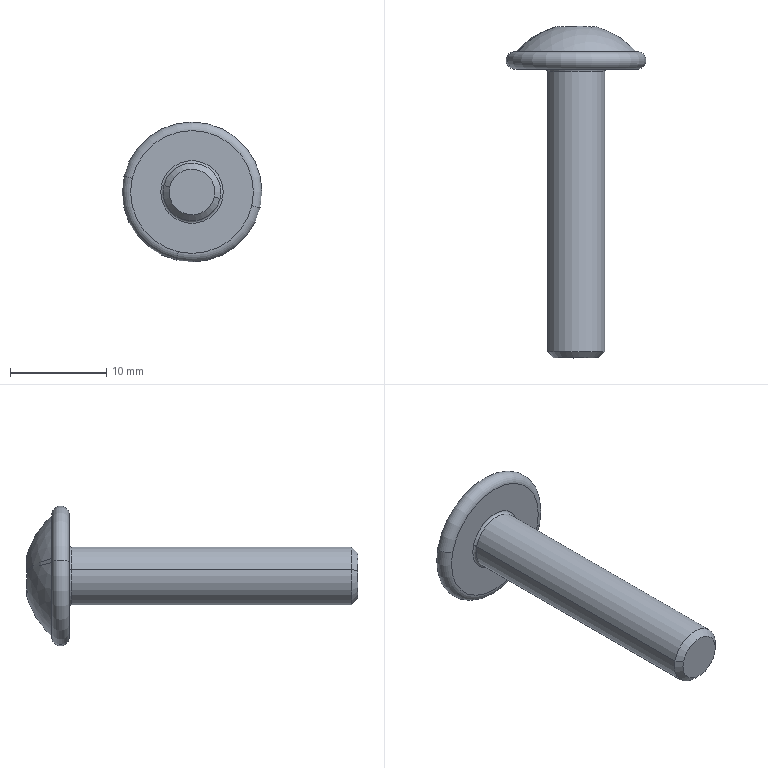Part | SolidWorks | features BaseBody 1 | 1 solid | 32 faces | box 14.55 x 34.479 x 14.55 mm | volume 1284 mm3 | cylinder 17 | torus 5 | sphere 4 | plane 4 | cone 2 | commonest cylinder face diameters 1.32 x6 3.14 x4 1 x3 1.26 x2 6 x2
STEP:
#1=CARTESIAN_POINT('',(1914.278,173.093,821.946));
#2=VERTEX_POINT('',#1);
#3=CARTESIAN_POINT('',(1913.973,173.055,822.157));
#4=VERTEX_POINT('',#3);
#5=CARTESIAN_POINT('',(1914.278,173.093,821.946));
#6=CARTESIAN_POINT('',(1914.154,173.093,821.975));
#7=CARTESIAN_POINT('',(1914.043,173.079,822.052));
#8=CARTESIAN_POINT('',(1913.973,173.055,822.157));
#9=B_SPLINE_CURVE_WITH_KNOTS('',3,(#5,#6,#7,#8),.UNSPECIFIED.,.F.,.F.,(4,4),(0.0003802,0.00076),.UNSPECIFIED.);
#10=EDGE_CURVE('',#2,#4,#9,.T.);
#11=ORIENTED_EDGE('',*,*,#10,.F.);
#12=CARTESIAN_POINT('',(1914.278,170.764,821.946));
#13=VERTEX_POINT('',#12);
#14=CARTESIAN_POINT('',(1914.278,173.214,821.946));
#15=DIRECTION('',(0.,-1.,0.));
#16=VECTOR('',#15,1000.);
#17=LINE('',#14,#16);
#18=EDGE_CURVE('',#2,#13,#17,.T.);
#19=ORIENTED_EDGE('',*,*,#18,.T.);
#20=CARTESIAN_POINT('',(1913.973,170.764,822.157));
#21=VERTEX_POINT('',#20);
#22=CARTESIAN_POINT('',(1914.39,170.764,822.434));
#23=DIRECTION('',(0.,-1.,0.));
#24=DIRECTION('',(-0.8332,0.,-0.5529));
#25=AXIS2_PLACEMENT_3D('',#22,#23,#24);
#26=CIRCLE('',#25,0.5);
#27=EDGE_CURVE('',#21,#13,#26,.T.);
#28=ORIENTED_EDGE('',*,*,#27,.F.);
#29=CARTESIAN_POINT('',(1913.973,170.764,822.157));
#30=DIRECTION('',(0.,1.,0.));
#31=VECTOR('',#30,1000.);
#32=LINE('',#29,#31);
#33=EDGE_CURVE('',#21,#4,#32,.T.);
#34=ORIENTED_EDGE('',*,*,#33,.T.);
#35=EDGE_LOOP('',(#11,#19,#28,#34));
#36=FACE_OUTER_BOUND('',#35,.T.);
#37=CARTESIAN_POINT('',(1914.39,173.214,822.434));
#38=DIRECTION('',(0.,-1.,0.));
#39=DIRECTION('',(-0.2239,0.,-0.9746));
#40=AXIS2_PLACEMENT_3D('',#37,#38,#39);
#41=CYLINDRICAL_SURFACE('',#40,0.5);
#42=ADVANCED_FACE('',(#36),#41,.T.);
#43=CARTESIAN_POINT('',(1912.656,172.978,818.453));
#44=VERTEX_POINT('',#43);
#45=CARTESIAN_POINT('',(1913.139,173.055,818.528));
#46=VERTEX_POINT('',#45);
#47=CARTESIAN_POINT('',(1912.656,172.978,818.453));
#48=CARTESIAN_POINT('',(1912.82,172.995,818.416));
#49=CARTESIAN_POINT('',(1912.995,173.023,818.443));
#50=CARTESIAN_POINT('',(1913.139,173.055,818.528));
#51=B_SPLINE_CURVE_WITH_KNOTS('',3,(#47,#48,#49,#50),.UNSPECIFIED.,.F.,.F.,(4,4),(0.0009315,0.001436),.UNSPECIFIED.);
#52=EDGE_CURVE('',#44,#46,#51,.T.);
#53=ORIENTED_EDGE('',*,*,#52,.F.);
#54=CARTESIAN_POINT('',(1912.656,170.764,818.453));
#55=VERTEX_POINT('',#54);
#56=CARTESIAN_POINT('',(1912.656,173.175,818.453));
#57=DIRECTION('',(0.,-1.,0.));
#58=VECTOR('',#57,1000.);
#59=LINE('',#56,#58);
#60=EDGE_CURVE('',#44,#55,#59,.T.);
#61=ORIENTED_EDGE('',*,*,#60,.T.);
#62=CARTESIAN_POINT('',(1913.139,170.764,818.528));
#63=VERTEX_POINT('',#62);
#64=CARTESIAN_POINT('',(1912.804,170.764,819.097));
#65=DIRECTION('',(0.,1.,0.));
#66=DIRECTION('',(0.5084,0.,-0.8611));
#67=AXIS2_PLACEMENT_3D('',#64,#65,#66);
#68=CIRCLE('',#67,0.66);
#69=EDGE_CURVE('',#63,#55,#68,.T.);
#70=ORIENTED_EDGE('',*,*,#69,.F.);
#71=CARTESIAN_POINT('',(1913.139,170.764,818.528));
#72=DIRECTION('',(0.,1.,0.));
#73=VECTOR('',#72,1000.);
#74=LINE('',#71,#73);
#75=EDGE_CURVE('',#63,#46,#74,.T.);
#76=ORIENTED_EDGE('',*,*,#75,.T.);
#77=EDGE_LOOP('',(#53,#61,#70,#76));
#78=FACE_OUTER_BOUND('',#77,.T.);
#79=CARTESIAN_POINT('',(1912.804,173.175,819.097));
#80=DIRECTION('',(0.,-1.,0.));
#81=DIRECTION('',(-0.2239,0.,-0.9746));
#82=AXIS2_PLACEMENT_3D('',#79,#80,#81);
#83=CYLINDRICAL_SURFACE('',#82,0.66);
#84=ADVANCED_FACE('',(#78),#83,.F.);
#85=CARTESIAN_POINT('',(1914.212,172.978,818.096));
#86=VERTEX_POINT('',#85);
#87=CARTESIAN_POINT('',(1914.972,173.009,818.492));
#88=VERTEX_POINT('',#87);
#89=CARTESIAN_POINT('',(1914.212,172.978,818.096));
#90=CARTESIAN_POINT('',(1914.363,172.962,818.061));
#91=CARTESIAN_POINT('',(1914.528,172.957,818.082));
#92=CARTESIAN_POINT('',(1914.804,172.968,818.226));
#93=CARTESIAN_POINT('',(1914.914,172.985,818.348));
#94=CARTESIAN_POINT('',(1914.972,173.009,818.492));
#95=B_SPLINE_CURVE_WITH_KNOTS('',3,(#89,#90,#91,#92,#93,#94),.UNSPECIFIED.,.F.,.F.,(4,2,4),(0.0005046,0.00097,0.001436),.UNSPECIFIED.);
#96=EDGE_CURVE('',#86,#88,#95,.T.);
#97=ORIENTED_EDGE('',*,*,#96,.F.);
#98=CARTESIAN_POINT('',(1914.212,170.764,818.096));
#99=VERTEX_POINT('',#98);
#100=CARTESIAN_POINT('',(1914.212,173.175,818.096));
#101=DIRECTION('',(0.,-1.,0.));
#102=VECTOR('',#101,1000.);
#103=LINE('',#100,#102);
#104=EDGE_CURVE('',#86,#99,#103,.T.);
#105=ORIENTED_EDGE('',*,*,#104,.T.);
#106=CARTESIAN_POINT('',(1914.972,170.764,818.492));
#107=VERTEX_POINT('',#106);
#108=CARTESIAN_POINT('',(1914.36,170.764,818.739));
#109=DIRECTION('',(0.,1.,0.));
#110=DIRECTION('',(0.9275,0.,-0.3739));
#111=AXIS2_PLACEMENT_3D('',#108,#109,#110);
#112=CIRCLE('',#111,0.66);
#113=EDGE_CURVE('',#107,#99,#112,.T.);
#114=ORIENTED_EDGE('',*,*,#113,.F.);
#115=CARTESIAN_POINT('',(1914.972,170.764,818.492));
#116=DIRECTION('',(0.,1.,0.));
#117=VECTOR('',#116,1000.);
#118=LINE('',#115,#117);
#119=EDGE_CURVE('',#107,#88,#118,.T.);
#120=ORIENTED_EDGE('',*,*,#119,.T.);
#121=EDGE_LOOP('',(#97,#105,#114,#120));
#122=FACE_OUTER_BOUND('',#121,.T.);
#123=CARTESIAN_POINT('',(1914.36,173.175,818.739));
#124=DIRECTION('',(0.,-1.,0.));
#125=DIRECTION('',(-0.2239,0.,-0.9746));
#126=AXIS2_PLACEMENT_3D('',#123,#124,#125);
#127=CYLINDRICAL_SURFACE('',#126,0.66);
#128=ADVANCED_FACE('',(#122),#127,.F.);
#129=CARTESIAN_POINT('',(1915.762,173.005,819.327));
#130=VERTEX_POINT('',#129);
#131=CARTESIAN_POINT('',(1916.054,172.959,819.608));
#132=VERTEX_POINT('',#131);
#133=CARTESIAN_POINT('',(1915.762,173.005,819.327));
#134=CARTESIAN_POINT('',(1915.887,172.983,819.386));
#135=CARTESIAN_POINT('',(1915.99,172.966,819.484));
#136=CARTESIAN_POINT('',(1916.054,172.959,819.608));
#137=B_SPLINE_CURVE_WITH_KNOTS('',3,(#133,#134,#135,#136),.UNSPECIFIED.,.F.,.F.,(4,4),(0.,0.0004132),.UNSPECIFIED.);
#138=EDGE_CURVE('',#130,#132,#137,.T.);
#139=ORIENTED_EDGE('',*,*,#138,.T.);
#140=CARTESIAN_POINT('',(1919.847,170.414,818.453));
#141=VERTEX_POINT('',#140);
#142=CARTESIAN_POINT('',(1913.892,165.077,820.266));
#143=DIRECTION('',(-0.2912,0.,-0.9567));
#144=DIRECTION('',(-0.9567,0.,0.2912));
#145=AXIS2_PLACEMENT_3D('',#142,#143,#144);
#146=CIRCLE('',#145,8.2);
#147=EDGE_CURVE('',#132,#141,#146,.T.);
#148=ORIENTED_EDGE('',*,*,#147,.T.);
#149=CARTESIAN_POINT('',(1907.825,170.414,821.659));
#150=VERTEX_POINT('',#149);
#151=CARTESIAN_POINT('',(1913.892,170.414,820.266));
#152=DIRECTION('',(0.,1.,0.));
#153=DIRECTION('',(0.9746,0.,-0.2239));
#154=AXIS2_PLACEMENT_3D('',#151,#152,#153);
#155=CIRCLE('',#154,6.225);
#156=EDGE_CURVE('',#141,#150,#155,.T.);
#157=ORIENTED_EDGE('',*,*,#156,.T.);
#158=CARTESIAN_POINT('',(1911.674,172.955,820.775));
#159=VERTEX_POINT('',#158);
#160=CARTESIAN_POINT('',(1913.892,165.077,820.266));
#161=DIRECTION('',(-0.2239,0.,-0.9746));
#162=DIRECTION('',(-0.7399,0.6509,0.1699));
#163=AXIS2_PLACEMENT_3D('',#160,#161,#162);
#164=CIRCLE('',#163,8.2);
#165=EDGE_CURVE('',#150,#159,#164,.T.);
#166=ORIENTED_EDGE('',*,*,#165,.T.);
#167=CARTESIAN_POINT('',(1911.799,173.005,820.237));
#168=VERTEX_POINT('',#167);
#169=CARTESIAN_POINT('',(1911.674,172.955,820.775));
#170=CARTESIAN_POINT('',(1911.631,172.955,820.587));
#171=CARTESIAN_POINT('',(1911.679,172.974,820.385));
#172=CARTESIAN_POINT('',(1911.799,173.005,820.237));
#173=B_SPLINE_CURVE_WITH_KNOTS('',3,(#169,#170,#171,#172),.UNSPECIFIED.,.F.,.F.,(4,4),(0.,0.0005707),.UNSPECIFIED.);
#174=EDGE_CURVE('',#159,#168,#173,.T.);
#175=ORIENTED_EDGE('',*,*,#174,.T.);
#176=CARTESIAN_POINT('',(1912.145,173.009,819.142));
#177=VERTEX_POINT('',#176);
#178=CARTESIAN_POINT('',(1911.799,173.005,820.237));
#179=CARTESIAN_POINT('',(1911.86,173.021,820.161));
#180=CARTESIAN_POINT('',(1911.914,173.033,820.08));
#181=CARTESIAN_POINT('',(1912.007,173.05,819.909));
#182=CARTESIAN_POINT('',(1912.046,173.054,819.817));
#183=CARTESIAN_POINT('',(1912.135,173.056,819.535));
#184=CARTESIAN_POINT('',(1912.159,173.04,819.338));
#185=CARTESIAN_POINT('',(1912.145,173.009,819.142));
#186=B_SPLINE_CURVE_WITH_KNOTS('',3,(#178,#179,#180,#181,#182,#183,#184,#185),.UNSPECIFIED.,.F.,.F.,(4,2,2,4),(0.,0.0002936,0.0005872,0.001174),.UNSPECIFIED.);
#187=EDGE_CURVE('',#168,#177,#186,.T.);
#188=ORIENTED_EDGE('',*,*,#187,.T.);
#189=CARTESIAN_POINT('',(1912.145,173.009,819.142));
#190=CARTESIAN_POINT('',(1912.135,172.985,818.987));
#191=CARTESIAN_POINT('',(1912.18,172.968,818.83));
#192=CARTESIAN_POINT('',(1912.366,172.957,818.578));
#193=CARTESIAN_POINT('',(1912.505,172.962,818.488));
#194=CARTESIAN_POINT('',(1912.656,172.978,818.453));
#195=B_SPLINE_CURVE_WITH_KNOTS('',3,(#189,#190,#191,#192,#193,#194),.UNSPECIFIED.,.F.,.F.,(4,2,4),(0.,0.0004658,0.0009315),.UNSPECIFIED.);
#196=EDGE_CURVE('',#177,#44,#195,.T.);
#197=ORIENTED_EDGE('',*,*,#196,.T.);
#198=ORIENTED_EDGE('',*,*,#52,.T.);
#199=CARTESIAN_POINT('',(1913.81,173.055,818.374));
#200=VERTEX_POINT('',#199);
#201=CARTESIAN_POINT('',(1913.139,173.055,818.528));
#202=CARTESIAN_POINT('',(1913.248,173.079,818.593));
#203=CARTESIAN_POINT('',(1913.382,173.093,818.614));
#204=CARTESIAN_POINT('',(1913.629,173.093,818.557));
#205=CARTESIAN_POINT('',(1913.74,173.079,818.479));
#206=CARTESIAN_POINT('',(1913.81,173.055,818.374));
#207=B_SPLINE_CURVE_WITH_KNOTS('',3,(#201,#202,#203,#204,#205,#206),.UNSPECIFIED.,.F.,.F.,(4,2,4),(0.,0.00038,0.00076),.UNSPECIFIED.);
#208=EDGE_CURVE('',#46,#200,#207,.T.);
#209=ORIENTED_EDGE('',*,*,#208,.T.);
#210=CARTESIAN_POINT('',(1913.81,173.055,818.374));
#211=CARTESIAN_POINT('',(1913.856,173.039,818.305));
#212=CARTESIAN_POINT('',(1913.915,173.024,818.245));
#213=CARTESIAN_POINT('',(1914.053,172.998,818.149));
#214=CARTESIAN_POINT('',(1914.13,172.986,818.115));
#215=CARTESIAN_POINT('',(1914.212,172.978,818.096));
#216=B_SPLINE_CURVE_WITH_KNOTS('',3,(#210,#211,#212,#213,#214,#215),.UNSPECIFIED.,.F.,.F.,(4,2,4),(0.,0.0002523,0.0005046),.UNSPECIFIED.);
#217=EDGE_CURVE('',#200,#86,#216,.T.);
#218=ORIENTED_EDGE('',*,*,#217,.T.);
#219=ORIENTED_EDGE('',*,*,#96,.T.);
#220=CARTESIAN_POINT('',(1914.972,173.009,818.492));
#221=CARTESIAN_POINT('',(1915.009,173.025,818.583));
#222=CARTESIAN_POINT('',(1915.054,173.036,818.67));
#223=CARTESIAN_POINT('',(1915.159,173.051,818.834));
#224=CARTESIAN_POINT('',(1915.22,173.055,818.913));
#225=CARTESIAN_POINT('',(1915.423,173.054,819.127));
#226=CARTESIAN_POINT('',(1915.585,173.037,819.244));
#227=CARTESIAN_POINT('',(1915.762,173.005,819.327));
#228=B_SPLINE_CURVE_WITH_KNOTS('',3,(#220,#221,#222,#223,#224,#225,#226,#227),.UNSPECIFIED.,.F.,.F.,(4,2,2,4),(0.,0.0002936,0.0005872,0.001174),.UNSPECIFIED.);
#229=EDGE_CURVE('',#88,#130,#228,.T.);
#230=ORIENTED_EDGE('',*,*,#229,.T.);
#231=EDGE_LOOP('',(#139,#148,#157,#166,#175,#188,#197,#198,#209,#218,#219,#230));
#232=FACE_OUTER_BOUND('',#231,.T.);
#233=CARTESIAN_POINT('',(1913.892,165.077,820.266));
#234=DIRECTION('',(-0.2912,0.,-0.9567));
#235=DIRECTION('',(-0.9567,0.,0.2912));
#236=AXIS2_PLACEMENT_3D('',#233,#234,#235);
#237=SPHERICAL_SURFACE('',#236,8.2);
#238=ADVANCED_FACE('',(#232),#237,.T.);
#239=CARTESIAN_POINT('',(1912.021,173.005,821.204));
#240=VERTEX_POINT('',#239);
#241=CARTESIAN_POINT('',(1911.729,172.959,820.924));
#242=VERTEX_POINT('',#241);
#243=CARTESIAN_POINT('',(1912.021,173.005,821.204));
#244=CARTESIAN_POINT('',(1911.896,172.983,821.146));
#245=CARTESIAN_POINT('',(1911.793,172.966,821.047));
#246=CARTESIAN_POINT('',(1911.729,172.959,820.924));
#247=B_SPLINE_CURVE_WITH_KNOTS('',3,(#243,#244,#245,#246),.UNSPECIFIED.,.F.,.F.,(4,4),(0.,0.0004132),.UNSPECIFIED.);
#248=EDGE_CURVE('',#240,#242,#247,.T.);
#249=ORIENTED_EDGE('',*,*,#248,.T.);
#250=CARTESIAN_POINT('',(1907.936,170.414,822.078));
#251=VERTEX_POINT('',#250);
#252=CARTESIAN_POINT('',(1913.892,165.077,820.266));
#253=DIRECTION('',(0.2912,0.,0.9567));
#254=DIRECTION('',(0.9567,0.,-0.2912));
#255=AXIS2_PLACEMENT_3D('',#252,#253,#254);
#256=CIRCLE('',#255,8.2);
#257=EDGE_CURVE('',#242,#251,#256,.T.);
#258=ORIENTED_EDGE('',*,*,#257,.T.);
#259=CARTESIAN_POINT('',(1919.959,170.414,818.872));
#260=VERTEX_POINT('',#259);
#261=CARTESIAN_POINT('',(1913.892,170.414,820.266));
#262=DIRECTION('',(0.,-1.,0.));
#263=DIRECTION('',(0.9746,0.,-0.2239));
#264=AXIS2_PLACEMENT_3D('',#261,#262,#263);
#265=CIRCLE('',#264,6.225);
#266=EDGE_CURVE('',#260,#251,#265,.T.);
#267=ORIENTED_EDGE('',*,*,#266,.F.);
#268=CARTESIAN_POINT('',(1916.109,172.955,819.756));
#269=VERTEX_POINT('',#268);
#270=CARTESIAN_POINT('',(1913.892,165.077,820.266));
#271=DIRECTION('',(-0.2239,0.,-0.9746));
#272=DIRECTION('',(0.7399,0.6509,-0.1699));
#273=AXIS2_PLACEMENT_3D('',#270,#271,#272);
#274=CIRCLE('',#273,8.2);
#275=EDGE_CURVE('',#269,#260,#274,.T.);
#276=ORIENTED_EDGE('',*,*,#275,.F.);
#277=CARTESIAN_POINT('',(1915.984,173.005,820.294));
#278=VERTEX_POINT('',#277);
#279=CARTESIAN_POINT('',(1916.109,172.955,819.756));
#280=CARTESIAN_POINT('',(1916.152,172.955,819.945));
#281=CARTESIAN_POINT('',(1916.104,172.974,820.146));
#282=CARTESIAN_POINT('',(1915.984,173.005,820.294));
#283=B_SPLINE_CURVE_WITH_KNOTS('',3,(#279,#280,#281,#282),.UNSPECIFIED.,.F.,.F.,(4,4),(0.,0.0005707),.UNSPECIFIED.);
#284=EDGE_CURVE('',#269,#278,#283,.T.);
#285=ORIENTED_EDGE('',*,*,#284,.T.);
#286=CARTESIAN_POINT('',(1915.638,173.009,821.39));
#287=VERTEX_POINT('',#286);
#288=CARTESIAN_POINT('',(1915.984,173.005,820.294));
#289=CARTESIAN_POINT('',(1915.923,173.021,820.37));
#290=CARTESIAN_POINT('',(1915.869,173.033,820.451));
#291=CARTESIAN_POINT('',(1915.776,173.05,820.623));
#292=CARTESIAN_POINT('',(1915.737,173.054,820.715));
#293=CARTESIAN_POINT('',(1915.648,173.056,820.996));
#294=CARTESIAN_POINT('',(1915.624,173.04,821.194));
#295=CARTESIAN_POINT('',(1915.638,173.009,821.39));
#296=B_SPLINE_CURVE_WITH_KNOTS('',3,(#288,#289,#290,#291,#292,#293,#294,#295),.UNSPECIFIED.,.F.,.F.,(4,2,2,4),(0.,0.0002936,0.0005872,0.001174),.UNSPECIFIED.);
#297=EDGE_CURVE('',#278,#287,#296,.T.);
#298=ORIENTED_EDGE('',*,*,#297,.T.);
#299=CARTESIAN_POINT('',(1914.644,173.055,822.003));
#300=VERTEX_POINT('',#299);
#301=CARTESIAN_POINT('',(1915.638,173.009,821.39));
#302=CARTESIAN_POINT('',(1915.646,172.991,821.509));
#303=CARTESIAN_POINT('',(1915.621,172.976,821.63));
#304=CARTESIAN_POINT('',(1915.512,172.96,821.842));
#305=CARTESIAN_POINT('',(1915.427,172.958,821.935));
#306=CARTESIAN_POINT('',(1915.222,172.968,822.06));
#307=CARTESIAN_POINT('',(1915.103,172.979,822.094));
#308=CARTESIAN_POINT('',(1914.864,173.012,822.096));
#309=CARTESIAN_POINT('',(1914.746,173.032,822.064));
#310=CARTESIAN_POINT('',(1914.644,173.055,822.003));
#311=B_SPLINE_CURVE_WITH_KNOTS('',3,(#301,#302,#303,#304,#305,#306,#307,#308,#309,#310),.UNSPECIFIED.,.F.,.F.,(4,2,2,2,4),(0.,0.0003589,0.0007178,0.001077,0.001436),.UNSPECIFIED.);
#312=EDGE_CURVE('',#287,#300,#311,.T.);
#313=ORIENTED_EDGE('',*,*,#312,.T.);
#314=CARTESIAN_POINT('',(1914.644,173.055,822.003));
#315=CARTESIAN_POINT('',(1914.535,173.079,821.939));
#316=CARTESIAN_POINT('',(1914.401,173.093,821.918));
#317=CARTESIAN_POINT('',(1914.278,173.093,821.946));
#318=B_SPLINE_CURVE_WITH_KNOTS('',3,(#314,#315,#316,#317),.UNSPECIFIED.,.F.,.F.,(4,4),(0.,0.0003802),.UNSPECIFIED.);
#319=EDGE_CURVE('',#300,#2,#318,.T.);
#320=ORIENTED_EDGE('',*,*,#319,.T.);
#321=ORIENTED_EDGE('',*,*,#10,.T.);
#322=CARTESIAN_POINT('',(1912.811,173.009,822.039));
#323=VERTEX_POINT('',#322);
#324=CARTESIAN_POINT('',(1913.973,173.055,822.157));
#325=CARTESIAN_POINT('',(1913.907,173.032,822.257));
#326=CARTESIAN_POINT('',(1913.815,173.012,822.336));
#327=CARTESIAN_POINT('',(1913.601,172.979,822.439));
#328=CARTESIAN_POINT('',(1913.478,172.968,822.461));
#329=CARTESIAN_POINT('',(1913.239,172.958,822.437));
#330=CARTESIAN_POINT('',(1913.123,172.96,822.392));
#331=CARTESIAN_POINT('',(1912.931,172.976,822.248));
#332=CARTESIAN_POINT('',(1912.856,172.991,822.15));
#333=CARTESIAN_POINT('',(1912.811,173.009,822.039));
#334=B_SPLINE_CURVE_WITH_KNOTS('',3,(#324,#325,#326,#327,#328,#329,#330,#331,#332,#333),.UNSPECIFIED.,.F.,.F.,(4,2,2,2,4),(0.,0.0003589,0.0007178,0.001077,0.001436),.UNSPECIFIED.);
#335=EDGE_CURVE('',#4,#323,#334,.T.);
#336=ORIENTED_EDGE('',*,*,#335,.T.);
#337=CARTESIAN_POINT('',(1912.811,173.009,822.039));
#338=CARTESIAN_POINT('',(1912.774,173.025,821.948));
#339=CARTESIAN_POINT('',(1912.729,173.036,821.862));
#340=CARTESIAN_POINT('',(1912.624,173.051,821.697));
#341=CARTESIAN_POINT('',(1912.563,173.055,821.618));
#342=CARTESIAN_POINT('',(1912.36,173.054,821.404));
#343=CARTESIAN_POINT('',(1912.198,173.037,821.288));
#344=CARTESIAN_POINT('',(1912.021,173.005,821.204));
#345=B_SPLINE_CURVE_WITH_KNOTS('',3,(#337,#338,#339,#340,#341,#342,#343,#344),.UNSPECIFIED.,.F.,.F.,(4,2,2,4),(0.,0.0002936,0.0005872,0.001174),.UNSPECIFIED.);
#346=EDGE_CURVE('',#323,#240,#345,.T.);
#347=ORIENTED_EDGE('',*,*,#346,.T.);
#348=EDGE_LOOP('',(#249,#258,#267,#276,#285,#298,#313,#320,#321,#336,#347));
#349=FACE_OUTER_BOUND('',#348,.T.);
#350=CARTESIAN_POINT('',(1913.892,165.077,820.266));
#351=DIRECTION('',(0.2912,0.,0.9567));
#352=DIRECTION('',(0.9567,0.,-0.2912));
#353=AXIS2_PLACEMENT_3D('',#350,#351,#352);
#354=SPHERICAL_SURFACE('',#353,8.2);
#355=ADVANCED_FACE('',(#349),#354,.T.);
#356=CARTESIAN_POINT('',(1912.464,170.414,814.053));
#357=VERTEX_POINT('',#356);
#358=CARTESIAN_POINT('',(1907.678,170.414,821.693));
#359=VERTEX_POINT('',#358);
#360=CARTESIAN_POINT('',(1913.892,170.414,820.266));
#361=DIRECTION('',(0.,1.,0.));
#362=DIRECTION('',(0.9746,0.,-0.2239));
#363=AXIS2_PLACEMENT_3D('',#360,#361,#362);
#364=CIRCLE('',#363,6.375);
#365=EDGE_CURVE('',#357,#359,#364,.T.);
#366=ORIENTED_EDGE('',*,*,#365,.F.);
#367=CARTESIAN_POINT('',(1912.464,168.614,814.053));
#368=VERTEX_POINT('',#367);
#369=CARTESIAN_POINT('',(1912.464,169.514,814.053));
#370=DIRECTION('',(-0.9746,0.,0.2239));
#371=DIRECTION('',(0.2239,0.,0.9746));
#372=AXIS2_PLACEMENT_3D('',#369,#370,#371);
#373=CIRCLE('',#372,0.9);
#374=EDGE_CURVE('',#357,#368,#373,.T.);
#375=ORIENTED_EDGE('',*,*,#374,.T.);
#376=CARTESIAN_POINT('',(1907.678,168.614,821.693));
#377=VERTEX_POINT('',#376);
#378=CARTESIAN_POINT('',(1913.892,168.614,820.266));
#379=DIRECTION('',(0.,1.,0.));
#380=DIRECTION('',(0.9746,0.,-0.2239));
#381=AXIS2_PLACEMENT_3D('',#378,#379,#380);
#382=CIRCLE('',#381,6.375);
#383=EDGE_CURVE('',#368,#377,#382,.T.);
#384=ORIENTED_EDGE('',*,*,#383,.T.);
#385=CARTESIAN_POINT('',(1907.678,169.514,821.693));
#386=DIRECTION('',(0.2239,0.,0.9746));
#387=DIRECTION('',(0.,-1.,0.));
#388=AXIS2_PLACEMENT_3D('',#385,#386,#387);
#389=CIRCLE('',#388,0.9);
#390=EDGE_CURVE('',#359,#377,#389,.T.);
#391=ORIENTED_EDGE('',*,*,#390,.F.);
#392=EDGE_LOOP('',(#366,#375,#384,#391));
#393=FACE_OUTER_BOUND('',#392,.T.);
#394=CARTESIAN_POINT('',(1913.892,169.514,820.266));
#395=DIRECTION('',(0.,-1.,0.));
#396=DIRECTION('',(-0.2239,0.,-0.9746));
#397=AXIS2_PLACEMENT_3D('',#394,#395,#396);
#398=TOROIDAL_SURFACE('',#397,6.375,0.9);
#399=ADVANCED_FACE('',(#393),#398,.T.);
#400=CARTESIAN_POINT('',(1916.206,138.614,819.734));
#401=VERTEX_POINT('',#400);
#402=CARTESIAN_POINT('',(1911.577,138.614,820.797));
#403=VERTEX_POINT('',#402);
#404=CARTESIAN_POINT('',(1913.892,138.614,820.266));
#405=DIRECTION('',(0.,-1.,0.));
#406=DIRECTION('',(0.9746,0.,-0.2239));
#407=AXIS2_PLACEMENT_3D('',#404,#405,#406);
#408=CIRCLE('',#407,2.375);
#409=EDGE_CURVE('',#401,#403,#408,.T.);
#410=ORIENTED_EDGE('',*,*,#409,.T.);
#411=CARTESIAN_POINT('',(1913.892,138.614,820.266));
#412=DIRECTION('',(0.,-1.,0.));
#413=DIRECTION('',(-0.9746,0.,0.2239));
#414=AXIS2_PLACEMENT_3D('',#411,#412,#413);
#415=CIRCLE('',#414,2.375);
#416=EDGE_CURVE('',#403,#401,#415,.T.);
#417=ORIENTED_EDGE('',*,*,#416,.T.);
#418=EDGE_LOOP('',(#410,#417));
#419=FACE_OUTER_BOUND('',#418,.T.);
#420=CARTESIAN_POINT('',(1916.882,138.614,822.139));
#421=DIRECTION('',(0.,-1.,0.));
#422=DIRECTION('',(-0.9746,0.,0.2239));
#423=AXIS2_PLACEMENT_3D('',#420,#421,#422);
#424=PLANE('',#423);
#425=ADVANCED_FACE('',(#419),#424,.T.);
#426=CARTESIAN_POINT('',(1910.968,139.239,820.937));
#427=VERTEX_POINT('',#426);
#428=CARTESIAN_POINT('',(1911.577,138.614,820.797));
#429=DIRECTION('',(-0.6892,0.7071,0.1583));
#430=VECTOR('',#429,1000.);
#431=LINE('',#428,#430);
#432=EDGE_CURVE('',#403,#427,#431,.T.);
#433=ORIENTED_EDGE('',*,*,#432,.T.);
#434=CARTESIAN_POINT('',(1916.815,139.239,819.594));
#435=VERTEX_POINT('',#434);
#436=CARTESIAN_POINT('',(1913.892,139.239,820.266));
#437=DIRECTION('',(0.,-1.,0.));
#438=DIRECTION('',(-0.9746,0.,0.2239));
#439=AXIS2_PLACEMENT_3D('',#436,#437,#438);
#440=CIRCLE('',#439,3.);
#441=EDGE_CURVE('',#427,#435,#440,.T.);
#442=ORIENTED_EDGE('',*,*,#441,.T.);
#443=CARTESIAN_POINT('',(1916.206,138.614,819.734));
#444=DIRECTION('',(-0.6892,-0.7071,0.1583));
#445=VECTOR('',#444,1000.);
#446=LINE('',#443,#445);
#447=EDGE_CURVE('',#435,#401,#446,.T.);
#448=ORIENTED_EDGE('',*,*,#447,.T.);
#449=ORIENTED_EDGE('',*,*,#416,.F.);
#450=EDGE_LOOP('',(#433,#442,#448,#449));
#451=FACE_OUTER_BOUND('',#450,.T.);
#452=CARTESIAN_POINT('',(1913.892,139.324,820.266));
#453=DIRECTION('',(0.,1.,0.));
#454=DIRECTION('',(-0.9746,0.,0.2239));
#455=AXIS2_PLACEMENT_3D('',#452,#453,#454);
#456=CONICAL_SURFACE('',#455,3.085,0.7854);
#457=ADVANCED_FACE('',(#451),#456,.T.);
#458=ORIENTED_EDGE('',*,*,#447,.F.);
#459=CARTESIAN_POINT('',(1913.892,139.239,820.266));
#460=DIRECTION('',(0.,-1.,0.));
#461=DIRECTION('',(0.9746,0.,-0.2239));
#462=AXIS2_PLACEMENT_3D('',#459,#460,#461);
#463=CIRCLE('',#462,3.);
#464=EDGE_CURVE('',#435,#427,#463,.T.);
#465=ORIENTED_EDGE('',*,*,#464,.T.);
#466=ORIENTED_EDGE('',*,*,#432,.F.);
#467=ORIENTED_EDGE('',*,*,#409,.F.);
#468=EDGE_LOOP('',(#458,#465,#466,#467));
#469=FACE_OUTER_BOUND('',#468,.T.);
#470=CARTESIAN_POINT('',(1913.892,139.324,820.266));
#471=DIRECTION('',(0.,1.,0.));
#472=DIRECTION('',(-0.9746,0.,0.2239));
#473=AXIS2_PLACEMENT_3D('',#470,#471,#472);
#474=CONICAL_SURFACE('',#473,3.085,0.7854);
#475=ADVANCED_FACE('',(#469),#474,.T.);
#476=CARTESIAN_POINT('',(1910.968,168.364,820.937));
#477=VERTEX_POINT('',#476);
#478=CARTESIAN_POINT('',(1910.968,168.364,820.937));
#479=DIRECTION('',(0.,1.,0.));
#480=VECTOR('',#479,1000.);
#481=LINE('',#478,#480);
#482=EDGE_CURVE('',#427,#477,#481,.T.);
#483=ORIENTED_EDGE('',*,*,#482,.F.);
#484=ORIENTED_EDGE('',*,*,#464,.F.);
#485=CARTESIAN_POINT('',(1916.815,168.364,819.594));
#486=VERTEX_POINT('',#485);
#487=CARTESIAN_POINT('',(1916.815,168.364,819.594));
#488=DIRECTION('',(0.,-1.,0.));
#489=VECTOR('',#488,1000.);
#490=LINE('',#487,#489);
#491=EDGE_CURVE('',#486,#435,#490,.T.);
#492=ORIENTED_EDGE('',*,*,#491,.F.);
#493=CARTESIAN_POINT('',(1913.892,168.364,820.266));
#494=DIRECTION('',(0.,-1.,0.));
#495=DIRECTION('',(0.9746,0.,-0.2239));
#496=AXIS2_PLACEMENT_3D('',#493,#494,#495);
#497=CIRCLE('',#496,3.);
#498=EDGE_CURVE('',#486,#477,#497,.T.);
#499=ORIENTED_EDGE('',*,*,#498,.T.);
#500=EDGE_LOOP('',(#483,#484,#492,#499));
#501=FACE_OUTER_BOUND('',#500,.T.);
#502=CARTESIAN_POINT('',(1913.892,168.947,820.266));
#503=DIRECTION('',(0.,-1.,0.));
#504=DIRECTION('',(0.9746,0.,-0.2239));
#505=AXIS2_PLACEMENT_3D('',#502,#503,#504);
#506=CYLINDRICAL_SURFACE('',#505,3.);
#507=ADVANCED_FACE('',(#501),#506,.T.);
#508=CARTESIAN_POINT('',(1910.724,168.614,820.993));
#509=VERTEX_POINT('',#508);
#510=CARTESIAN_POINT('',(1910.724,168.364,820.993));
#511=DIRECTION('',(0.2239,0.,0.9746));
#512=DIRECTION('',(0.000000004,1.,-0.000000001));
#513=AXIS2_PLACEMENT_3D('',#510,#511,#512);
#514=CIRCLE('',#513,0.25);
#515=EDGE_CURVE('',#477,#509,#514,.T.);
#516=ORIENTED_EDGE('',*,*,#515,.F.);
#517=ORIENTED_EDGE('',*,*,#498,.F.);
#518=CARTESIAN_POINT('',(1917.059,168.614,819.538));
#519=VERTEX_POINT('',#518);
#520=CARTESIAN_POINT('',(1917.059,168.364,819.538));
#521=DIRECTION('',(0.2239,0.,0.9746));
#522=DIRECTION('',(-0.000000004,1.,0.000000001));
#523=AXIS2_PLACEMENT_3D('',#520,#521,#522);
#524=CIRCLE('',#523,0.25);
#525=EDGE_CURVE('',#519,#486,#524,.T.);
#526=ORIENTED_EDGE('',*,*,#525,.F.);
#527=CARTESIAN_POINT('',(1913.892,168.614,820.266));
#528=DIRECTION('',(0.,-1.,0.));
#529=DIRECTION('',(0.9746,0.,-0.2239));
#530=AXIS2_PLACEMENT_3D('',#527,#528,#529);
#531=CIRCLE('',#530,3.25);
#532=EDGE_CURVE('',#519,#509,#531,.T.);
#533=ORIENTED_EDGE('',*,*,#532,.T.);
#534=EDGE_LOOP('',(#516,#517,#526,#533));
#535=FACE_OUTER_BOUND('',#534,.T.);
#536=CARTESIAN_POINT('',(1913.892,168.364,820.266));
#537=DIRECTION('',(0.,-1.,0.));
#538=DIRECTION('',(0.9746,0.,-0.2239));
#539=AXIS2_PLACEMENT_3D('',#536,#537,#538);
#540=TOROIDAL_SURFACE('',#539,3.25,0.25);
#541=ADVANCED_FACE('',(#535),#540,.F.);
#542=CARTESIAN_POINT('',(1920.105,168.614,818.839));
#543=VERTEX_POINT('',#542);
#544=CARTESIAN_POINT('',(1913.892,168.614,820.266));
#545=DIRECTION('',(0.,1.,0.));
#546=DIRECTION('',(0.9746,0.,-0.2239));
#547=AXIS2_PLACEMENT_3D('',#544,#545,#546);
#548=CIRCLE('',#547,6.375);
#549=EDGE_CURVE('',#543,#368,#548,.T.);
#550=ORIENTED_EDGE('',*,*,#549,.F.);
#551=CARTESIAN_POINT('',(1913.892,168.614,820.266));
#552=DIRECTION('',(0.,-1.,0.));
#553=DIRECTION('',(0.9746,0.,-0.2239));
#554=AXIS2_PLACEMENT_3D('',#551,#552,#553);
#555=CIRCLE('',#554,6.375);
#556=EDGE_CURVE('',#543,#377,#555,.T.);
#557=ORIENTED_EDGE('',*,*,#556,.T.);
#558=ORIENTED_EDGE('',*,*,#383,.F.);
#559=EDGE_LOOP('',(#550,#557,#558));
#560=FACE_OUTER_BOUND('',#559,.T.);
#561=CARTESIAN_POINT('',(1913.892,168.614,820.266));
#562=DIRECTION('',(0.,-1.,0.));
#563=DIRECTION('',(-0.9746,0.,0.2239));
#564=AXIS2_PLACEMENT_3D('',#561,#562,#563);
#565=CIRCLE('',#564,3.25);
#566=EDGE_CURVE('',#509,#519,#565,.T.);
#567=ORIENTED_EDGE('',*,*,#566,.F.);
#568=ORIENTED_EDGE('',*,*,#532,.F.);
#569=EDGE_LOOP('',(#567,#568));
#570=FACE_BOUND('',#569,.T.);
#571=CARTESIAN_POINT('',(1921.842,168.614,825.262));
#572=DIRECTION('',(0.,-1.,0.));
#573=DIRECTION('',(-0.9746,0.,0.2239));
#574=AXIS2_PLACEMENT_3D('',#571,#572,#573);
#575=PLANE('',#574);
#576=ADVANCED_FACE('',(#560,#570),#575,.T.);
#577=CARTESIAN_POINT('',(1920.105,170.414,818.839));
#578=VERTEX_POINT('',#577);
#579=CARTESIAN_POINT('',(1913.892,170.414,820.266));
#580=DIRECTION('',(0.,-1.,0.));
#581=DIRECTION('',(0.9746,0.,-0.2239));
#582=AXIS2_PLACEMENT_3D('',#579,#580,#581);
#583=CIRCLE('',#582,6.375);
#584=EDGE_CURVE('',#578,#359,#583,.T.);
#585=ORIENTED_EDGE('',*,*,#584,.T.);
#586=ORIENTED_EDGE('',*,*,#390,.T.);
#587=ORIENTED_EDGE('',*,*,#556,.F.);
#588=CARTESIAN_POINT('',(1920.105,169.514,818.839));
#589=DIRECTION('',(0.2239,0.,0.9746));
#590=DIRECTION('',(0.,-1.,0.));
#591=AXIS2_PLACEMENT_3D('',#588,#589,#590);
#592=CIRCLE('',#591,0.9);
#593=EDGE_CURVE('',#543,#578,#592,.T.);
#594=ORIENTED_EDGE('',*,*,#593,.T.);
#595=EDGE_LOOP('',(#585,#586,#587,#594));
#596=FACE_OUTER_BOUND('',#595,.T.);
#597=CARTESIAN_POINT('',(1913.892,169.514,820.266));
#598=DIRECTION('',(0.,-1.,0.));
#599=DIRECTION('',(-0.2239,0.,-0.9746));
#600=AXIS2_PLACEMENT_3D('',#597,#598,#599);
#601=TOROIDAL_SURFACE('',#600,6.375,0.9);
#602=ADVANCED_FACE('',(#596),#601,.T.);
#603=ORIENTED_EDGE('',*,*,#374,.F.);
#604=CARTESIAN_POINT('',(1913.892,170.414,820.266));
#605=DIRECTION('',(0.,1.,0.));
#606=DIRECTION('',(0.9746,0.,-0.2239));
#607=AXIS2_PLACEMENT_3D('',#604,#605,#606);
#608=CIRCLE('',#607,6.375);
#609=EDGE_CURVE('',#578,#357,#608,.T.);
#610=ORIENTED_EDGE('',*,*,#609,.F.);
#611=ORIENTED_EDGE('',*,*,#593,.F.);
#612=ORIENTED_EDGE('',*,*,#549,.T.);
#613=EDGE_LOOP('',(#603,#610,#611,#612));
#614=FACE_OUTER_BOUND('',#613,.T.);
#615=CARTESIAN_POINT('',(1913.892,169.514,820.266));
#616=DIRECTION('',(0.,-1.,0.));
#617=DIRECTION('',(-0.2239,0.,-0.9746));
#618=AXIS2_PLACEMENT_3D('',#615,#616,#617);
#619=TOROIDAL_SURFACE('',#618,6.375,0.9);
#620=ADVANCED_FACE('',(#614),#619,.T.);
#621=ORIENTED_EDGE('',*,*,#584,.F.);
#622=ORIENTED_EDGE('',*,*,#609,.T.);
#623=ORIENTED_EDGE('',*,*,#365,.T.);
#624=EDGE_LOOP('',(#621,#622,#623));
#625=FACE_OUTER_BOUND('',#624,.T.);
#626=CARTESIAN_POINT('',(1913.892,170.414,820.266));
#627=DIRECTION('',(0.,1.,0.));
#628=DIRECTION('',(0.9746,0.,-0.2239));
#629=AXIS2_PLACEMENT_3D('',#626,#627,#628);
#630=CIRCLE('',#629,6.225);
#631=EDGE_CURVE('',#260,#141,#630,.T.);
#632=ORIENTED_EDGE('',*,*,#631,.F.);
#633=ORIENTED_EDGE('',*,*,#266,.T.);
#634=CARTESIAN_POINT('',(1913.892,170.414,820.266));
#635=DIRECTION('',(0.,-1.,0.));
#636=DIRECTION('',(0.9746,0.,-0.2239));
#637=AXIS2_PLACEMENT_3D('',#634,#635,#636);
#638=CIRCLE('',#637,6.225);
#639=EDGE_CURVE('',#251,#150,#638,.T.);
#640=ORIENTED_EDGE('',*,*,#639,.T.);
#641=ORIENTED_EDGE('',*,*,#156,.F.);
#642=EDGE_LOOP('',(#632,#633,#640,#641));
#643=FACE_BOUND('',#642,.T.);
#644=CARTESIAN_POINT('',(1921.842,170.414,825.262));
#645=DIRECTION('',(0.,1.,0.));
#646=DIRECTION('',(-0.2239,0.,-0.9746));
#647=AXIS2_PLACEMENT_3D('',#644,#645,#646);
#648=PLANE('',#647);
#649=ADVANCED_FACE('',(#625,#643),#648,.T.);
#650=ORIENTED_EDGE('',*,*,#257,.F.);
#651=CARTESIAN_POINT('',(1911.729,172.959,820.924));
#652=CARTESIAN_POINT('',(1911.705,172.956,820.877));
#653=CARTESIAN_POINT('',(1911.686,172.955,820.827));
#654=CARTESIAN_POINT('',(1911.674,172.955,820.775));
#655=B_SPLINE_CURVE_WITH_KNOTS('',3,(#651,#652,#653,#654),.UNSPECIFIED.,.F.,.F.,(4,4),(0.0004132,0.0005707),.UNSPECIFIED.);
#656=EDGE_CURVE('',#242,#159,#655,.T.);
#657=ORIENTED_EDGE('',*,*,#656,.T.);
#658=ORIENTED_EDGE('',*,*,#165,.F.);
#659=ORIENTED_EDGE('',*,*,#639,.F.);
#660=EDGE_LOOP('',(#650,#657,#658,#659));
#661=FACE_OUTER_BOUND('',#660,.T.);
#662=CARTESIAN_POINT('',(1913.892,165.077,820.266));
#663=DIRECTION('',(0.2912,0.,0.9567));
#664=DIRECTION('',(0.9567,0.,-0.2912));
#665=AXIS2_PLACEMENT_3D('',#662,#663,#664);
#666=SPHERICAL_SURFACE('',#665,8.2);
#667=ADVANCED_FACE('',(#661),#666,.T.);
#668=CARTESIAN_POINT('',(1911.799,170.764,820.237));
#669=VERTEX_POINT('',#668);
#670=CARTESIAN_POINT('',(1912.021,170.764,821.204));
#671=VERTEX_POINT('',#670);
#672=CARTESIAN_POINT('',(1912.288,170.764,820.634));
#673=DIRECTION('',(0.,1.,0.));
#674=DIRECTION('',(-0.7769,0.,-0.6296));
#675=AXIS2_PLACEMENT_3D('',#672,#673,#674);
#676=CIRCLE('',#675,0.63);
#677=EDGE_CURVE('',#669,#671,#676,.T.);
#678=ORIENTED_EDGE('',*,*,#677,.F.);
#679=CARTESIAN_POINT('',(1911.799,170.764,820.237));
#680=DIRECTION('',(0.,1.,0.));
#681=VECTOR('',#680,1000.);
#682=LINE('',#679,#681);
#683=EDGE_CURVE('',#669,#168,#682,.T.);
#684=ORIENTED_EDGE('',*,*,#683,.T.);
#685=ORIENTED_EDGE('',*,*,#174,.F.);
#686=ORIENTED_EDGE('',*,*,#656,.F.);
#687=ORIENTED_EDGE('',*,*,#248,.F.);
#688=CARTESIAN_POINT('',(1912.021,170.764,821.204));
#689=DIRECTION('',(0.,1.,0.));
#690=VECTOR('',#689,1000.);
#691=LINE('',#688,#690);
#692=EDGE_CURVE('',#671,#240,#691,.T.);
#693=ORIENTED_EDGE('',*,*,#692,.F.);
#694=EDGE_LOOP('',(#678,#684,#685,#686,#687,#693));
#695=FACE_OUTER_BOUND('',#694,.T.);
#696=CARTESIAN_POINT('',(1912.288,173.125,820.634));
#697=DIRECTION('',(0.,-1.,0.));
#698=DIRECTION('',(-0.2239,0.,-0.9746));
#699=AXIS2_PLACEMENT_3D('',#696,#697,#698);
#700=CYLINDRICAL_SURFACE('',#699,0.63);
#701=ADVANCED_FACE('',(#695),#700,.F.);
#702=ORIENTED_EDGE('',*,*,#346,.F.);
#703=CARTESIAN_POINT('',(1912.811,170.764,822.039));
#704=VERTEX_POINT('',#703);
#705=CARTESIAN_POINT('',(1912.811,170.764,822.039));
#706=DIRECTION('',(0.,1.,0.));
#707=VECTOR('',#706,1000.);
#708=LINE('',#705,#707);
#709=EDGE_CURVE('',#704,#323,#708,.T.);
#710=ORIENTED_EDGE('',*,*,#709,.F.);
#711=CARTESIAN_POINT('',(1911.355,170.764,822.626));
#712=DIRECTION('',(0.,-1.,0.));
#713=DIRECTION('',(0.4243,0.,-0.9055));
#714=AXIS2_PLACEMENT_3D('',#711,#712,#713);
#715=CIRCLE('',#714,1.57);
#716=EDGE_CURVE('',#671,#704,#715,.T.);
#717=ORIENTED_EDGE('',*,*,#716,.F.);
#718=ORIENTED_EDGE('',*,*,#692,.T.);
#719=EDGE_LOOP('',(#702,#710,#717,#718));
#720=FACE_OUTER_BOUND('',#719,.T.);
#721=CARTESIAN_POINT('',(1911.355,173.175,822.626));
#722=DIRECTION('',(0.,-1.,0.));
#723=DIRECTION('',(-0.2239,0.,-0.9746));
#724=AXIS2_PLACEMENT_3D('',#721,#722,#723);
#725=CYLINDRICAL_SURFACE('',#724,1.57);
#726=ADVANCED_FACE('',(#720),#725,.T.);
#727=ORIENTED_EDGE('',*,*,#716,.T.);
#728=CARTESIAN_POINT('',(1913.423,170.764,821.792));
#729=DIRECTION('',(0.,1.,0.));
#730=DIRECTION('',(-0.9275,0.,0.3739));
#731=AXIS2_PLACEMENT_3D('',#728,#729,#730);
#732=CIRCLE('',#731,0.66);
#733=EDGE_CURVE('',#704,#21,#732,.T.);
#734=ORIENTED_EDGE('',*,*,#733,.T.);
#735=ORIENTED_EDGE('',*,*,#27,.T.);
#736=CARTESIAN_POINT('',(1914.644,170.764,822.003));
#737=VERTEX_POINT('',#736);
#738=CARTESIAN_POINT('',(1914.39,170.764,822.434));
#739=DIRECTION('',(0.,-1.,0.));
#740=DIRECTION('',(-0.8332,0.,-0.5529));
#741=AXIS2_PLACEMENT_3D('',#738,#739,#740);
#742=CIRCLE('',#741,0.5);
#743=EDGE_CURVE('',#13,#737,#742,.T.);
#744=ORIENTED_EDGE('',*,*,#743,.T.);
#745=CARTESIAN_POINT('',(1915.638,170.764,821.39));
#746=VERTEX_POINT('',#745);
#747=CARTESIAN_POINT('',(1914.979,170.764,821.435));
#748=DIRECTION('',(0.,1.,0.));
#749=DIRECTION('',(-0.5084,0.,0.8611));
#750=AXIS2_PLACEMENT_3D('',#747,#748,#749);
#751=CIRCLE('',#750,0.66);
#752=EDGE_CURVE('',#737,#746,#751,.T.);
#753=ORIENTED_EDGE('',*,*,#752,.T.);
#754=CARTESIAN_POINT('',(1915.984,170.764,820.294));
#755=VERTEX_POINT('',#754);
#756=CARTESIAN_POINT('',(1917.204,170.764,821.283));
#757=DIRECTION('',(0.,-1.,0.));
#758=DIRECTION('',(-0.9977,0.,0.06829));
#759=AXIS2_PLACEMENT_3D('',#756,#757,#758);
#760=CIRCLE('',#759,1.57);
#761=EDGE_CURVE('',#746,#755,#760,.T.);
#762=ORIENTED_EDGE('',*,*,#761,.T.);
#763=CARTESIAN_POINT('',(1915.762,170.764,819.327));
#764=VERTEX_POINT('',#763);
#765=CARTESIAN_POINT('',(1915.495,170.764,819.898));
#766=DIRECTION('',(0.,1.,0.));
#767=DIRECTION('',(0.7769,0.,0.6296));
#768=AXIS2_PLACEMENT_3D('',#765,#766,#767);
#769=CIRCLE('',#768,0.63);
#770=EDGE_CURVE('',#755,#764,#769,.T.);
#771=ORIENTED_EDGE('',*,*,#770,.T.);
#772=CARTESIAN_POINT('',(1916.428,170.764,817.905));
#773=DIRECTION('',(0.,-1.,0.));
#774=DIRECTION('',(-0.4243,0.,0.9055));
#775=AXIS2_PLACEMENT_3D('',#772,#773,#774);
#776=CIRCLE('',#775,1.57);
#777=EDGE_CURVE('',#764,#107,#776,.T.);
#778=ORIENTED_EDGE('',*,*,#777,.T.);
#779=ORIENTED_EDGE('',*,*,#113,.T.);
#780=CARTESIAN_POINT('',(1913.81,170.764,818.374));
#781=VERTEX_POINT('',#780);
#782=CARTESIAN_POINT('',(1914.36,170.764,818.739));
#783=DIRECTION('',(0.,1.,0.));
#784=DIRECTION('',(0.9275,0.,-0.3739));
#785=AXIS2_PLACEMENT_3D('',#782,#783,#784);
#786=CIRCLE('',#785,0.66);
#787=EDGE_CURVE('',#99,#781,#786,.T.);
#788=ORIENTED_EDGE('',*,*,#787,.T.);
#789=CARTESIAN_POINT('',(1913.394,170.764,818.098));
#790=DIRECTION('',(0.,-1.,0.));
#791=DIRECTION('',(0.8332,0.,0.5529));
#792=AXIS2_PLACEMENT_3D('',#789,#790,#791);
#793=CIRCLE('',#792,0.5);
#794=EDGE_CURVE('',#781,#63,#793,.T.);
#795=ORIENTED_EDGE('',*,*,#794,.T.);
#796=ORIENTED_EDGE('',*,*,#69,.T.);
#797=CARTESIAN_POINT('',(1912.145,170.764,819.142));
#798=VERTEX_POINT('',#797);
#799=CARTESIAN_POINT('',(1912.804,170.764,819.097));
#800=DIRECTION('',(0.,1.,0.));
#801=DIRECTION('',(0.5084,0.,-0.8611));
#802=AXIS2_PLACEMENT_3D('',#799,#800,#801);
#803=CIRCLE('',#802,0.66);
#804=EDGE_CURVE('',#55,#798,#803,.T.);
#805=ORIENTED_EDGE('',*,*,#804,.T.);
#806=CARTESIAN_POINT('',(1910.579,170.764,819.249));
#807=DIRECTION('',(0.,-1.,0.));
#808=DIRECTION('',(0.9977,0.,-0.06829));
#809=AXIS2_PLACEMENT_3D('',#806,#807,#808);
#810=CIRCLE('',#809,1.57);
#811=EDGE_CURVE('',#798,#669,#810,.T.);
#812=ORIENTED_EDGE('',*,*,#811,.T.);
#813=ORIENTED_EDGE('',*,*,#677,.T.);
#814=EDGE_LOOP('',(#727,#734,#735,#744,#753,#762,#771,#778,#779,#788,#795,#796,#805,#812,#813));
#815=FACE_OUTER_BOUND('',#814,.T.);
#816=CARTESIAN_POINT('',(1916.717,170.764,821.839));
#817=DIRECTION('',(0.,1.,0.));
#818=DIRECTION('',(-0.2239,0.,-0.9746));
#819=AXIS2_PLACEMENT_3D('',#816,#817,#818);
#820=PLANE('',#819);
#821=ADVANCED_FACE('',(#815),#820,.T.);
#822=ORIENTED_EDGE('',*,*,#811,.F.);
#823=CARTESIAN_POINT('',(1912.145,170.764,819.142));
#824=DIRECTION('',(0.,1.,0.));
#825=VECTOR('',#824,1000.);
#826=LINE('',#823,#825);
#827=EDGE_CURVE('',#798,#177,#826,.T.);
#828=ORIENTED_EDGE('',*,*,#827,.T.);
#829=ORIENTED_EDGE('',*,*,#187,.F.);
#830=ORIENTED_EDGE('',*,*,#683,.F.);
#831=EDGE_LOOP('',(#822,#828,#829,#830));
#832=FACE_OUTER_BOUND('',#831,.T.);
#833=CARTESIAN_POINT('',(1910.579,173.175,819.249));
#834=DIRECTION('',(0.,-1.,0.));
#835=DIRECTION('',(-0.2239,0.,-0.9746));
#836=AXIS2_PLACEMENT_3D('',#833,#834,#835);
#837=CYLINDRICAL_SURFACE('',#836,1.57);
#838=ADVANCED_FACE('',(#832),#837,.T.);
#839=ORIENTED_EDGE('',*,*,#147,.F.);
#840=CARTESIAN_POINT('',(1916.054,172.959,819.608));
#841=CARTESIAN_POINT('',(1916.079,172.956,819.655));
#842=CARTESIAN_POINT('',(1916.097,172.955,819.705));
#843=CARTESIAN_POINT('',(1916.109,172.955,819.756));
#844=B_SPLINE_CURVE_WITH_KNOTS('',3,(#840,#841,#842,#843),.UNSPECIFIED.,.F.,.F.,(4,4),(0.0004132,0.0005707),.UNSPECIFIED.);
#845=EDGE_CURVE('',#132,#269,#844,.T.);
#846=ORIENTED_EDGE('',*,*,#845,.T.);
#847=ORIENTED_EDGE('',*,*,#275,.T.);
#848=ORIENTED_EDGE('',*,*,#631,.T.);
#849=EDGE_LOOP('',(#839,#846,#847,#848));
#850=FACE_OUTER_BOUND('',#849,.T.);
#851=CARTESIAN_POINT('',(1913.892,165.077,820.266));
#852=DIRECTION('',(-0.2912,0.,-0.9567));
#853=DIRECTION('',(-0.9567,0.,0.2912));
#854=AXIS2_PLACEMENT_3D('',#851,#852,#853);
#855=SPHERICAL_SURFACE('',#854,8.2);
#856=ADVANCED_FACE('',(#850),#855,.T.);
#857=ORIENTED_EDGE('',*,*,#770,.F.);
#858=CARTESIAN_POINT('',(1915.984,170.764,820.294));
#859=DIRECTION('',(0.,1.,0.));
#860=VECTOR('',#859,1000.);
#861=LINE('',#858,#860);
#862=EDGE_CURVE('',#755,#278,#861,.T.);
#863=ORIENTED_EDGE('',*,*,#862,.T.);
#864=ORIENTED_EDGE('',*,*,#284,.F.);
#865=ORIENTED_EDGE('',*,*,#845,.F.);
#866=ORIENTED_EDGE('',*,*,#138,.F.);
#867=CARTESIAN_POINT('',(1915.762,170.764,819.327));
#868=DIRECTION('',(0.,1.,0.));
#869=VECTOR('',#868,1000.);
#870=LINE('',#867,#869);
#871=EDGE_CURVE('',#764,#130,#870,.T.);
#872=ORIENTED_EDGE('',*,*,#871,.F.);
#873=EDGE_LOOP('',(#857,#863,#864,#865,#866,#872));
#874=FACE_OUTER_BOUND('',#873,.T.);
#875=CARTESIAN_POINT('',(1915.495,173.125,819.898));
#876=DIRECTION('',(0.,-1.,0.));
#877=DIRECTION('',(-0.2239,0.,-0.9746));
#878=AXIS2_PLACEMENT_3D('',#875,#876,#877);
#879=CYLINDRICAL_SURFACE('',#878,0.63);
#880=ADVANCED_FACE('',(#874),#879,.F.);
#881=ORIENTED_EDGE('',*,*,#777,.F.);
#882=ORIENTED_EDGE('',*,*,#871,.T.);
#883=ORIENTED_EDGE('',*,*,#229,.F.);
#884=ORIENTED_EDGE('',*,*,#119,.F.);
#885=EDGE_LOOP('',(#881,#882,#883,#884));
#886=FACE_OUTER_BOUND('',#885,.T.);
#887=CARTESIAN_POINT('',(1916.428,173.175,817.905));
#888=DIRECTION('',(0.,-1.,0.));
#889=DIRECTION('',(-0.2239,0.,-0.9746));
#890=AXIS2_PLACEMENT_3D('',#887,#888,#889);
#891=CYLINDRICAL_SURFACE('',#890,1.57);
#892=ADVANCED_FACE('',(#886),#891,.T.);
#893=ORIENTED_EDGE('',*,*,#104,.F.);
#894=ORIENTED_EDGE('',*,*,#217,.F.);
#895=CARTESIAN_POINT('',(1913.81,170.764,818.374));
#896=DIRECTION('',(0.,1.,0.));
#897=VECTOR('',#896,1000.);
#898=LINE('',#895,#897);
#899=EDGE_CURVE('',#781,#200,#898,.T.);
#900=ORIENTED_EDGE('',*,*,#899,.F.);
#901=ORIENTED_EDGE('',*,*,#787,.F.);
#902=EDGE_LOOP('',(#893,#894,#900,#901));
#903=FACE_OUTER_BOUND('',#902,.T.);
#904=CARTESIAN_POINT('',(1914.36,173.175,818.739));
#905=DIRECTION('',(0.,-1.,0.));
#906=DIRECTION('',(-0.2239,0.,-0.9746));
#907=AXIS2_PLACEMENT_3D('',#904,#905,#906);
#908=CYLINDRICAL_SURFACE('',#907,0.66);
#909=ADVANCED_FACE('',(#903),#908,.F.);
#910=ORIENTED_EDGE('',*,*,#794,.F.);
#911=ORIENTED_EDGE('',*,*,#899,.T.);
#912=ORIENTED_EDGE('',*,*,#208,.F.);
#913=ORIENTED_EDGE('',*,*,#75,.F.);
#914=EDGE_LOOP('',(#910,#911,#912,#913));
#915=FACE_OUTER_BOUND('',#914,.T.);
#916=CARTESIAN_POINT('',(1913.394,173.214,818.098));
#917=DIRECTION('',(0.,-1.,0.));
#918=DIRECTION('',(-0.2239,0.,-0.9746));
#919=AXIS2_PLACEMENT_3D('',#916,#917,#918);
#920=CYLINDRICAL_SURFACE('',#919,0.5);
#921=ADVANCED_FACE('',(#915),#920,.T.);
#922=ORIENTED_EDGE('',*,*,#60,.F.);
#923=ORIENTED_EDGE('',*,*,#196,.F.);
#924=ORIENTED_EDGE('',*,*,#827,.F.);
#925=ORIENTED_EDGE('',*,*,#804,.F.);
#926=EDGE_LOOP('',(#922,#923,#924,#925));
#927=FACE_OUTER_BOUND('',#926,.T.);
#928=CARTESIAN_POINT('',(1912.804,173.175,819.097));
#929=DIRECTION('',(0.,-1.,0.));
#930=DIRECTION('',(-0.2239,0.,-0.9746));
#931=AXIS2_PLACEMENT_3D('',#928,#929,#930);
#932=CYLINDRICAL_SURFACE('',#931,0.66);
#933=ADVANCED_FACE('',(#927),#932,.F.);
#934=ORIENTED_EDGE('',*,*,#761,.F.);
#935=CARTESIAN_POINT('',(1915.638,170.764,821.39));
#936=DIRECTION('',(0.,1.,0.));
#937=VECTOR('',#936,1000.);
#938=LINE('',#935,#937);
#939=EDGE_CURVE('',#746,#287,#938,.T.);
#940=ORIENTED_EDGE('',*,*,#939,.T.);
#941=ORIENTED_EDGE('',*,*,#297,.F.);
#942=ORIENTED_EDGE('',*,*,#862,.F.);
#943=EDGE_LOOP('',(#934,#940,#941,#942));
#944=FACE_OUTER_BOUND('',#943,.T.);
#945=CARTESIAN_POINT('',(1917.204,173.175,821.283));
#946=DIRECTION('',(0.,-1.,0.));
#947=DIRECTION('',(-0.2239,0.,-0.9746));
#948=AXIS2_PLACEMENT_3D('',#945,#946,#947);
#949=CYLINDRICAL_SURFACE('',#948,1.57);
#950=ADVANCED_FACE('',(#944),#949,.T.);
#951=ORIENTED_EDGE('',*,*,#752,.F.);
#952=CARTESIAN_POINT('',(1914.644,170.764,822.003));
#953=DIRECTION('',(0.,1.,0.));
#954=VECTOR('',#953,1000.);
#955=LINE('',#952,#954);
#956=EDGE_CURVE('',#737,#300,#955,.T.);
#957=ORIENTED_EDGE('',*,*,#956,.T.);
#958=ORIENTED_EDGE('',*,*,#312,.F.);
#959=ORIENTED_EDGE('',*,*,#939,.F.);
#960=EDGE_LOOP('',(#951,#957,#958,#959));
#961=FACE_OUTER_BOUND('',#960,.T.);
#962=CARTESIAN_POINT('',(1914.979,173.175,821.435));
#963=DIRECTION('',(0.,-1.,0.));
#964=DIRECTION('',(-0.2239,0.,-0.9746));
#965=AXIS2_PLACEMENT_3D('',#962,#963,#964);
#966=CYLINDRICAL_SURFACE('',#965,0.66);
#967=ADVANCED_FACE('',(#961),#966,.F.);
#968=ORIENTED_EDGE('',*,*,#18,.F.);
#969=ORIENTED_EDGE('',*,*,#319,.F.);
#970=ORIENTED_EDGE('',*,*,#956,.F.);
#971=ORIENTED_EDGE('',*,*,#743,.F.);
#972=EDGE_LOOP('',(#968,#969,#970,#971));
#973=FACE_OUTER_BOUND('',#972,.T.);
#974=CARTESIAN_POINT('',(1914.39,173.214,822.434));
#975=DIRECTION('',(0.,-1.,0.));
#976=DIRECTION('',(-0.2239,0.,-0.9746));
#977=AXIS2_PLACEMENT_3D('',#974,#975,#976);
#978=CYLINDRICAL_SURFACE('',#977,0.5);
#979=ADVANCED_FACE('',(#973),#978,.T.);
#980=ORIENTED_EDGE('',*,*,#733,.F.);
#981=ORIENTED_EDGE('',*,*,#709,.T.);
#982=ORIENTED_EDGE('',*,*,#335,.F.);
#983=ORIENTED_EDGE('',*,*,#33,.F.);
#984=EDGE_LOOP('',(#980,#981,#982,#983));
#985=FACE_OUTER_BOUND('',#984,.T.);
#986=CARTESIAN_POINT('',(1913.423,173.175,821.792));
#987=DIRECTION('',(0.,-1.,0.));
#988=DIRECTION('',(-0.2239,0.,-0.9746));
#989=AXIS2_PLACEMENT_3D('',#986,#987,#988);
#990=CYLINDRICAL_SURFACE('',#989,0.66);
#991=ADVANCED_FACE('',(#985),#990,.F.);
#992=ORIENTED_EDGE('',*,*,#525,.T.);
#993=CARTESIAN_POINT('',(1913.892,168.364,820.266));
#994=DIRECTION('',(0.,-1.,0.));
#995=DIRECTION('',(-0.9746,0.,0.2239));
#996=AXIS2_PLACEMENT_3D('',#993,#994,#995);
#997=CIRCLE('',#996,3.);
#998=EDGE_CURVE('',#477,#486,#997,.T.);
#999=ORIENTED_EDGE('',*,*,#998,.F.);
#1000=ORIENTED_EDGE('',*,*,#515,.T.);
#1001=ORIENTED_EDGE('',*,*,#566,.T.);
#1002=EDGE_LOOP('',(#992,#999,#1000,#1001));
#1003=FACE_OUTER_BOUND('',#1002,.T.);
#1004=CARTESIAN_POINT('',(1913.892,168.364,820.266));
#1005=DIRECTION('',(0.,-1.,0.));
#1006=DIRECTION('',(0.9746,0.,-0.2239));
#1007=AXIS2_PLACEMENT_3D('',#1004,#1005,#1006);
#1008=TOROIDAL_SURFACE('',#1007,3.25,0.25);
#1009=ADVANCED_FACE('',(#1003),#1008,.F.);
#1010=ORIENTED_EDGE('',*,*,#491,.T.);
#1011=ORIENTED_EDGE('',*,*,#441,.F.);
#1012=ORIENTED_EDGE('',*,*,#482,.T.);
#1013=ORIENTED_EDGE('',*,*,#998,.T.);
#1014=EDGE_LOOP('',(#1010,#1011,#1012,#1013));
#1015=FACE_OUTER_BOUND('',#1014,.T.);
#1016=CARTESIAN_POINT('',(1913.892,168.947,820.266));
#1017=DIRECTION('',(0.,-1.,0.));
#1018=DIRECTION('',(0.9746,0.,-0.2239));
#1019=AXIS2_PLACEMENT_3D('',#1016,#1017,#1018);
#1020=CYLINDRICAL_SURFACE('',#1019,3.);
#1021=ADVANCED_FACE('',(#1015),#1020,.T.);
#1022=CLOSED_SHELL('',(#42,#84,#128,#238,#355,#399,#425,#457,#475,#507,#541,#576,#602,#620,#649,#667,#701,#726,#821,#838,#856,#880,#892,#909,#921,#933,#950,#967,#979,#991,#1009,#1021));
#1023=MANIFOLD_SOLID_BREP('',#1022);
#1024=CARTESIAN_POINT('',(0.,0.,0.));
#1025=DIRECTION('',(0.,0.,1.));
#1026=DIRECTION('',(1.,0.,0.));
#1027=AXIS2_PLACEMENT_3D('',#1024,#1025,#1026);
#1028=(LENGTH_UNIT()NAMED_UNIT(*)SI_UNIT(.MILLI.,.METRE.));
#1029=UNCERTAINTY_MEASURE_WITH_UNIT(LENGTH_MEASURE(0.00001),#1028,'','');
#1030=(NAMED_UNIT(*)PLANE_ANGLE_UNIT()SI_UNIT($,.RADIAN.));
#1031=(NAMED_UNIT(*)SI_UNIT($,.STERADIAN.)SOLID_ANGLE_UNIT());
#1032=(GEOMETRIC_REPRESENTATION_CONTEXT(3)GLOBAL_UNCERTAINTY_ASSIGNED_CONTEXT((#1029))GLOBAL_UNIT_ASSIGNED_CONTEXT((#1028,#1030,#1031))REPRESENTATION_CONTEXT('',''));
#1033=ADVANCED_BREP_SHAPE_REPRESENTATION('',(#1023,#1027),#1032);